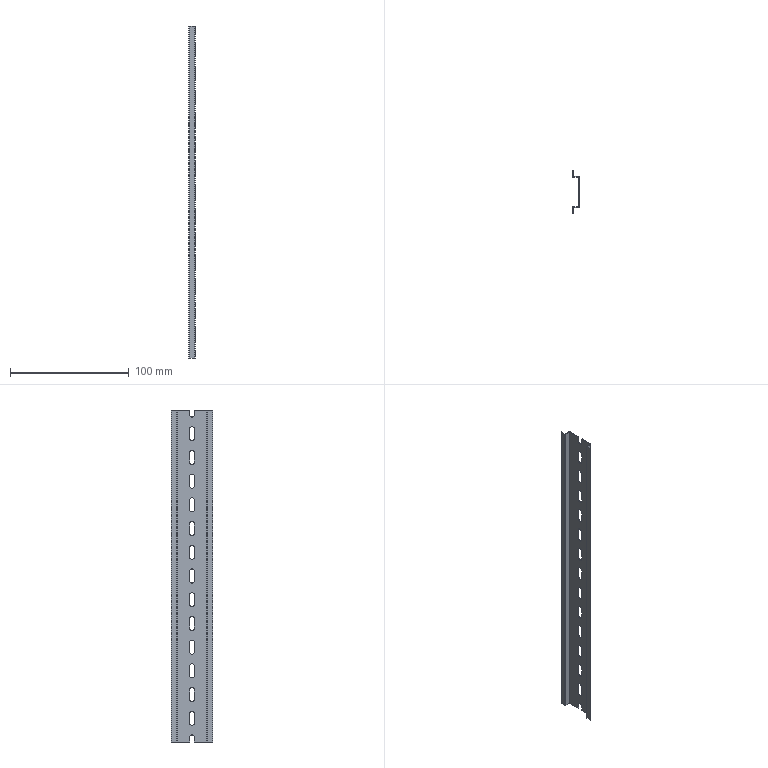Part | STEP file | 1 solid | 98 faces | box 5.5 x 35 x 280 mm | volume 5866 mm3 | plane 62 | cylinder 36 | commonest cylinder face diameters 4.2 x28 0.4 x4 1.4 x4